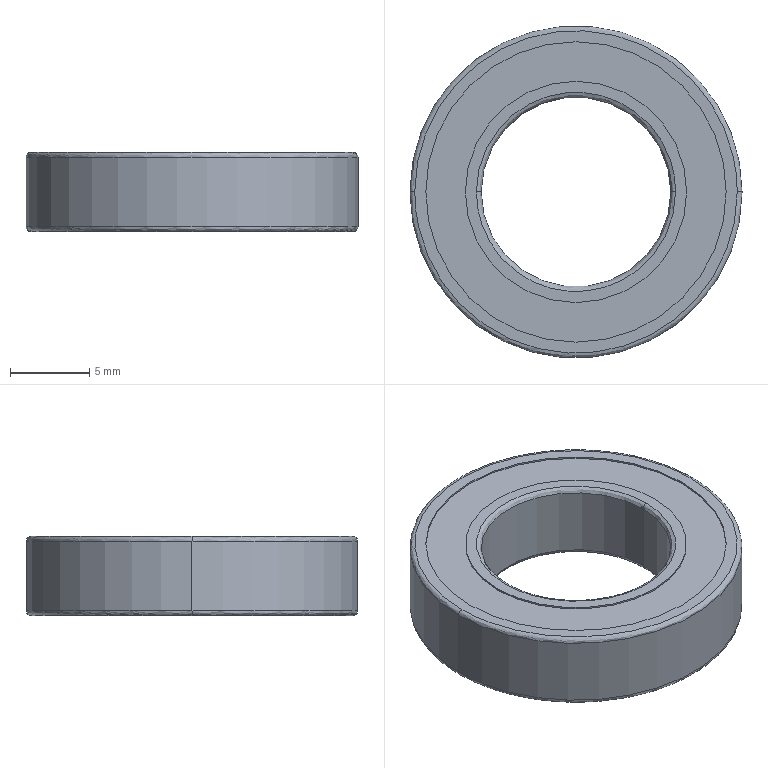Part | SolidWorks | features BaseBody 1 | 1 solid | 26 faces | box 21 x 21 x 5 mm | volume 1137 mm3 | cylinder 12 | spline 8 | plane 6 | commonest cylinder face diameters 14 x4 19 x4 12 x2 21 x2
STEP:
#1=CARTESIAN_POINT('',(-10.2,0.,-5.));
#2=VERTEX_POINT('',#1);
#3=CARTESIAN_POINT('',(10.2,0.,-5.));
#4=VERTEX_POINT('',#3);
#5=CARTESIAN_POINT('',(-10.2,0.,-5.));
#6=CARTESIAN_POINT('',(-10.2,-20.4,-5.));
#7=CARTESIAN_POINT('',(10.2,-20.4,-5.));
#8=CARTESIAN_POINT('',(10.2,0.,-5.));
#9=(BOUNDED_CURVE()B_SPLINE_CURVE(3,(#5,#6,#7,#8),.UNSPECIFIED.,.F.,.F.)B_SPLINE_CURVE_WITH_KNOTS((4,4),(0.,0.5),.UNSPECIFIED.)CURVE()GEOMETRIC_REPRESENTATION_ITEM()RATIONAL_B_SPLINE_CURVE((1.,0.3333,0.3333,1.))REPRESENTATION_ITEM(''));
#10=EDGE_CURVE('',#2,#4,#9,.T.);
#11=ORIENTED_EDGE('',*,*,#10,.T.);
#12=CARTESIAN_POINT('',(10.5,0.,-4.7));
#13=VERTEX_POINT('',#12);
#14=CARTESIAN_POINT('',(10.2,0.,-4.7));
#15=DIRECTION('',(0.,-1.,0.));
#16=DIRECTION('',(1.,0.,0.));
#17=AXIS2_PLACEMENT_3D('',#14,#15,#16);
#18=CIRCLE('',#17,0.3);
#19=EDGE_CURVE('',#4,#13,#18,.T.);
#20=ORIENTED_EDGE('',*,*,#19,.T.);
#21=CARTESIAN_POINT('',(-10.5,0.,-4.7));
#22=VERTEX_POINT('',#21);
#23=CARTESIAN_POINT('',(0.,0.,-4.7));
#24=DIRECTION('',(0.,0.,1.));
#25=DIRECTION('',(1.,0.,0.));
#26=AXIS2_PLACEMENT_3D('',#23,#24,#25);
#27=CIRCLE('',#26,10.5);
#28=EDGE_CURVE('',#22,#13,#27,.T.);
#29=ORIENTED_EDGE('',*,*,#28,.F.);
#30=CARTESIAN_POINT('',(-10.2,0.,-4.7));
#31=DIRECTION('',(0.,1.,0.));
#32=DIRECTION('',(-1.,0.,0.));
#33=AXIS2_PLACEMENT_3D('',#30,#31,#32);
#34=CIRCLE('',#33,0.3);
#35=EDGE_CURVE('',#2,#22,#34,.T.);
#36=ORIENTED_EDGE('',*,*,#35,.F.);
#37=EDGE_LOOP('',(#11,#20,#29,#36));
#38=FACE_OUTER_BOUND('',#37,.T.);
#39=CARTESIAN_POINT('',(10.2,0.,-5.));
#40=CARTESIAN_POINT('',(10.2,-20.4,-5.));
#41=CARTESIAN_POINT('',(-10.2,-20.4,-5.));
#42=CARTESIAN_POINT('',(-10.2,0.,-5.));
#43=CARTESIAN_POINT('',(10.376,0.,-5.));
#44=CARTESIAN_POINT('',(10.376,-20.751,-5.));
#45=CARTESIAN_POINT('',(-10.376,-20.751,-5.));
#46=CARTESIAN_POINT('',(-10.376,0.,-5.));
#47=CARTESIAN_POINT('',(10.5,0.,-4.876));
#48=CARTESIAN_POINT('',(10.5,-21.,-4.876));
#49=CARTESIAN_POINT('',(-10.5,-21.,-4.876));
#50=CARTESIAN_POINT('',(-10.5,0.,-4.876));
#51=CARTESIAN_POINT('',(10.5,0.,-4.7));
#52=CARTESIAN_POINT('',(10.5,-21.,-4.7));
#53=CARTESIAN_POINT('',(-10.5,-21.,-4.7));
#54=CARTESIAN_POINT('',(-10.5,0.,-4.7));
#55=(BOUNDED_SURFACE()B_SPLINE_SURFACE(3,3,((#39,#40,#41,#42),(#43,#44,#45,#46),(#47,#48,#49,#50),(#51,#52,#53,#54)),.UNSPECIFIED.,.F.,.F.,.F.)B_SPLINE_SURFACE_WITH_KNOTS((4,4),(4,4),(0.,1.),(0.,1.),.UNSPECIFIED.)GEOMETRIC_REPRESENTATION_ITEM()RATIONAL_B_SPLINE_SURFACE(((1.,0.3333,0.3333,1.),(0.8047,0.2682,0.2682,0.8047),(0.8047,0.2682,0.2682,0.8047),(1.,0.3333,0.3333,1.)))REPRESENTATION_ITEM('')SURFACE());
#56=ADVANCED_FACE('',(#38),#55,.T.);
#57=CARTESIAN_POINT('',(10.5,0.,-0.3));
#58=VERTEX_POINT('',#57);
#59=CARTESIAN_POINT('',(-10.5,0.,-0.3));
#60=VERTEX_POINT('',#59);
#61=CARTESIAN_POINT('',(0.,0.,-0.3));
#62=DIRECTION('',(0.,0.,-1.));
#63=DIRECTION('',(1.,0.,0.));
#64=AXIS2_PLACEMENT_3D('',#61,#62,#63);
#65=CIRCLE('',#64,10.5);
#66=EDGE_CURVE('',#58,#60,#65,.T.);
#67=ORIENTED_EDGE('',*,*,#66,.F.);
#68=CARTESIAN_POINT('',(10.2,0.,0.));
#69=VERTEX_POINT('',#68);
#70=CARTESIAN_POINT('',(10.2,0.,-0.3));
#71=DIRECTION('',(0.,-1.,0.));
#72=DIRECTION('',(1.,0.,0.));
#73=AXIS2_PLACEMENT_3D('',#70,#71,#72);
#74=CIRCLE('',#73,0.3);
#75=EDGE_CURVE('',#58,#69,#74,.T.);
#76=ORIENTED_EDGE('',*,*,#75,.T.);
#77=CARTESIAN_POINT('',(-10.2,0.,0.));
#78=VERTEX_POINT('',#77);
#79=CARTESIAN_POINT('',(10.2,0.,0.));
#80=CARTESIAN_POINT('',(10.2,-20.4,0.));
#81=CARTESIAN_POINT('',(-10.2,-20.4,0.));
#82=CARTESIAN_POINT('',(-10.2,0.,0.));
#83=(BOUNDED_CURVE()B_SPLINE_CURVE(3,(#79,#80,#81,#82),.UNSPECIFIED.,.F.,.F.)B_SPLINE_CURVE_WITH_KNOTS((4,4),(0.5,1.),.UNSPECIFIED.)CURVE()GEOMETRIC_REPRESENTATION_ITEM()RATIONAL_B_SPLINE_CURVE((1.,0.3333,0.3333,1.))REPRESENTATION_ITEM(''));
#84=EDGE_CURVE('',#69,#78,#83,.T.);
#85=ORIENTED_EDGE('',*,*,#84,.T.);
#86=CARTESIAN_POINT('',(-10.2,0.,-0.3));
#87=DIRECTION('',(0.,1.,0.));
#88=DIRECTION('',(-1.,0.,0.));
#89=AXIS2_PLACEMENT_3D('',#86,#87,#88);
#90=CIRCLE('',#89,0.3);
#91=EDGE_CURVE('',#60,#78,#90,.T.);
#92=ORIENTED_EDGE('',*,*,#91,.F.);
#93=EDGE_LOOP('',(#67,#76,#85,#92));
#94=FACE_OUTER_BOUND('',#93,.T.);
#95=CARTESIAN_POINT('',(10.5,0.,-0.3));
#96=CARTESIAN_POINT('',(10.5,-21.,-0.3));
#97=CARTESIAN_POINT('',(-10.5,-21.,-0.3));
#98=CARTESIAN_POINT('',(-10.5,0.,-0.3));
#99=CARTESIAN_POINT('',(10.5,0.,-0.1243));
#100=CARTESIAN_POINT('',(10.5,-21.,-0.1243));
#101=CARTESIAN_POINT('',(-10.5,-21.,-0.1243));
#102=CARTESIAN_POINT('',(-10.5,0.,-0.1243));
#103=CARTESIAN_POINT('',(10.376,0.,0.));
#104=CARTESIAN_POINT('',(10.376,-20.751,0.));
#105=CARTESIAN_POINT('',(-10.376,-20.751,0.));
#106=CARTESIAN_POINT('',(-10.376,0.,0.));
#107=CARTESIAN_POINT('',(10.2,0.,0.));
#108=CARTESIAN_POINT('',(10.2,-20.4,0.));
#109=CARTESIAN_POINT('',(-10.2,-20.4,0.));
#110=CARTESIAN_POINT('',(-10.2,0.,0.));
#111=(BOUNDED_SURFACE()B_SPLINE_SURFACE(3,3,((#95,#96,#97,#98),(#99,#100,#101,#102),(#103,#104,#105,#106),(#107,#108,#109,#110)),.UNSPECIFIED.,.F.,.F.,.F.)B_SPLINE_SURFACE_WITH_KNOTS((4,4),(4,4),(0.,1.),(0.,1.),.UNSPECIFIED.)GEOMETRIC_REPRESENTATION_ITEM()RATIONAL_B_SPLINE_SURFACE(((1.,0.3333,0.3333,1.),(0.8047,0.2682,0.2682,0.8047),(0.8047,0.2682,0.2682,0.8047),(1.,0.3333,0.3333,1.)))REPRESENTATION_ITEM('')SURFACE());
#112=ADVANCED_FACE('',(#94),#111,.T.);
#113=CARTESIAN_POINT('',(-6.,0.,-4.7));
#114=VERTEX_POINT('',#113);
#115=CARTESIAN_POINT('',(6.,0.,-4.7));
#116=VERTEX_POINT('',#115);
#117=CARTESIAN_POINT('',(0.,0.,-4.7));
#118=DIRECTION('',(0.,0.,1.));
#119=DIRECTION('',(-1.,0.,0.));
#120=AXIS2_PLACEMENT_3D('',#117,#118,#119);
#121=CIRCLE('',#120,6.);
#122=EDGE_CURVE('',#114,#116,#121,.T.);
#123=ORIENTED_EDGE('',*,*,#122,.T.);
#124=CARTESIAN_POINT('',(6.3,0.,-5.));
#125=VERTEX_POINT('',#124);
#126=CARTESIAN_POINT('',(6.3,0.,-4.7));
#127=DIRECTION('',(0.,-1.,0.));
#128=DIRECTION('',(1.,0.,0.));
#129=AXIS2_PLACEMENT_3D('',#126,#127,#128);
#130=CIRCLE('',#129,0.3);
#131=EDGE_CURVE('',#116,#125,#130,.T.);
#132=ORIENTED_EDGE('',*,*,#131,.T.);
#133=CARTESIAN_POINT('',(-6.3,0.,-5.));
#134=VERTEX_POINT('',#133);
#135=CARTESIAN_POINT('',(-6.3,0.,-5.));
#136=CARTESIAN_POINT('',(-6.3,-0.1926,-5.));
#137=CARTESIAN_POINT('',(-6.287,-0.4803,-5.));
#138=CARTESIAN_POINT('',(-6.249,-0.814,-5.));
#139=CARTESIAN_POINT('',(-6.224,-0.9804,-5.));
#140=CARTESIAN_POINT('',(-6.212,-1.052,-5.));
#141=CARTESIAN_POINT('',(-6.203,-1.099,-5.));
#142=CARTESIAN_POINT('',(-6.199,-1.121,-5.));
#143=CARTESIAN_POINT('',(-6.158,-1.347,-5.));
#144=CARTESIAN_POINT('',(-6.088,-1.644,-5.));
#145=CARTESIAN_POINT('',(-5.981,-1.984,-5.));
#146=CARTESIAN_POINT('',(-5.93,-2.128,-5.));
#147=CARTESIAN_POINT('',(-5.895,-2.224,-5.));
#148=CARTESIAN_POINT('',(-5.877,-2.27,-5.));
#149=CARTESIAN_POINT('',(-5.779,-2.517,-5.));
#150=CARTESIAN_POINT('',(-5.648,-2.806,-5.));
#151=CARTESIAN_POINT('',(-5.494,-3.085,-5.));
#152=CARTESIAN_POINT('',(-5.387,-3.268,-5.));
#153=CARTESIAN_POINT('',(-5.333,-3.356,-5.));
#154=CARTESIAN_POINT('',(-5.035,-3.811,-5.));
#155=CARTESIAN_POINT('',(-4.762,-4.147,-5.));
#156=CARTESIAN_POINT('',(-4.301,-4.608,-5.));
#157=CARTESIAN_POINT('',(-4.06,-4.826,-5.));
#158=CARTESIAN_POINT('',(-3.76,-5.057,-5.));
#159=CARTESIAN_POINT('',(-3.627,-5.151,-5.));
#160=CARTESIAN_POINT('',(-3.538,-5.213,-5.));
#161=CARTESIAN_POINT('',(-3.492,-5.244,-5.));
#162=CARTESIAN_POINT('',(-3.269,-5.389,-5.));
#163=CARTESIAN_POINT('',(-2.995,-5.55,-5.));
#164=CARTESIAN_POINT('',(-2.661,-5.712,-5.));
#165=CARTESIAN_POINT('',(-2.516,-5.776,-5.));
#166=CARTESIAN_POINT('',(-2.418,-5.818,-5.));
#167=CARTESIAN_POINT('',(-2.366,-5.839,-5.));
#168=CARTESIAN_POINT('',(-2.129,-5.933,-5.));
#169=CARTESIAN_POINT('',(-1.84,-6.031,-5.));
#170=CARTESIAN_POINT('',(-1.496,-6.121,-5.));
#171=CARTESIAN_POINT('',(-1.322,-6.16,-5.));
#172=CARTESIAN_POINT('',(-1.247,-6.175,-5.));
#173=CARTESIAN_POINT('',(-1.197,-6.185,-5.));
#174=CARTESIAN_POINT('',(-1.17,-6.19,-5.));
#175=CARTESIAN_POINT('',(-0.7678,-6.265,-5.));
#176=CARTESIAN_POINT('',(-0.385,-6.3,-5.));
#177=CARTESIAN_POINT('',(0.1925,-6.3,-5.));
#178=CARTESIAN_POINT('',(0.4802,-6.287,-5.));
#179=CARTESIAN_POINT('',(0.8139,-6.249,-5.));
#180=CARTESIAN_POINT('',(0.9803,-6.224,-5.));
#181=CARTESIAN_POINT('',(1.051,-6.212,-5.));
#182=CARTESIAN_POINT('',(1.099,-6.203,-5.));
#183=CARTESIAN_POINT('',(1.121,-6.199,-5.));
#184=CARTESIAN_POINT('',(1.347,-6.158,-5.));
#185=CARTESIAN_POINT('',(1.644,-6.088,-5.));
#186=CARTESIAN_POINT('',(1.984,-5.981,-5.));
#187=CARTESIAN_POINT('',(2.128,-5.93,-5.));
#188=CARTESIAN_POINT('',(2.224,-5.895,-5.));
#189=CARTESIAN_POINT('',(2.27,-5.877,-5.));
#190=CARTESIAN_POINT('',(2.517,-5.779,-5.));
#191=CARTESIAN_POINT('',(2.806,-5.648,-5.));
#192=CARTESIAN_POINT('',(3.085,-5.494,-5.));
#193=CARTESIAN_POINT('',(3.268,-5.387,-5.));
#194=CARTESIAN_POINT('',(3.356,-5.333,-5.));
#195=CARTESIAN_POINT('',(3.811,-5.035,-5.));
#196=CARTESIAN_POINT('',(4.147,-4.762,-5.));
#197=CARTESIAN_POINT('',(4.608,-4.301,-5.));
#198=CARTESIAN_POINT('',(4.826,-4.06,-5.));
#199=CARTESIAN_POINT('',(5.057,-3.76,-5.));
#200=CARTESIAN_POINT('',(5.151,-3.627,-5.));
#201=CARTESIAN_POINT('',(5.213,-3.538,-5.));
#202=CARTESIAN_POINT('',(5.244,-3.492,-5.));
#203=CARTESIAN_POINT('',(5.389,-3.269,-5.));
#204=CARTESIAN_POINT('',(5.55,-2.995,-5.));
#205=CARTESIAN_POINT('',(5.712,-2.661,-5.));
#206=CARTESIAN_POINT('',(5.776,-2.516,-5.));
#207=CARTESIAN_POINT('',(5.818,-2.418,-5.));
#208=CARTESIAN_POINT('',(5.839,-2.366,-5.));
#209=CARTESIAN_POINT('',(5.933,-2.129,-5.));
#210=CARTESIAN_POINT('',(6.031,-1.84,-5.));
#211=CARTESIAN_POINT('',(6.121,-1.496,-5.));
#212=CARTESIAN_POINT('',(6.16,-1.322,-5.));
#213=CARTESIAN_POINT('',(6.175,-1.247,-5.));
#214=CARTESIAN_POINT('',(6.185,-1.197,-5.));
#215=CARTESIAN_POINT('',(6.19,-1.17,-5.));
#216=CARTESIAN_POINT('',(6.265,-0.7678,-5.));
#217=CARTESIAN_POINT('',(6.3,-0.385,-5.));
#218=CARTESIAN_POINT('',(6.3,0.,-5.));
#219=B_SPLINE_CURVE_WITH_KNOTS('',3,(#135,#136,#137,#138,#139,#140,#141,#142,#143,#144,#145,#146,#147,#148,#149,#150,#151,#152,#153,#154,#155,#156,#157,#158,#159,#160,#161,#162,#163,#164,#165,#166,#167,#168,#169,#170,#171,#172,#173,#174,#175,#176,#177,#178,#179,#180,#181,#182,#183,#184,#185,#186,#187,#188,#189,#190,#191,#192,#193,#194,#195,#196,#197,#198,#199,#200,#201,#202,#203,#204,#205,#206,#207,#208,#209,#210,#211,#212,#213,#214,#215,#216,#217,#218),.UNSPECIFIED.,.F.,.F.,(4,1,1,1,2,2,1,1,2,2,1,2,2,2,1,1,2,2,1,1,2,2,1,1,1,2,2,2,1,1,1,2,2,1,1,2,2,1,2,2,2,1,1,2,2,1,1,2,2,1,1,1,2,2,4),(0.,0.01563,0.02344,0.02734,0.0293,0.03125,0.04688,0.05469,0.05859,0.0625,0.07813,0.08594,0.09375,0.125,0.1406,0.1484,0.1523,0.1563,0.1719,0.1797,0.1836,0.1875,0.2031,0.2109,0.2148,0.2168,0.2188,0.25,0.2656,0.2734,0.2773,0.2793,0.2813,0.2969,0.3047,0.3086,0.3125,0.3281,0.3359,0.3438,0.375,0.3906,0.3984,0.4023,0.4063,0.4219,0.4297,0.4336,0.4375,0.4531,0.4609,0.4648,0.4668,0.4688,0.5),.UNSPECIFIED.);
#220=EDGE_CURVE('',#134,#125,#219,.T.);
#221=ORIENTED_EDGE('',*,*,#220,.F.);
#222=CARTESIAN_POINT('',(-6.3,0.,-4.7));
#223=DIRECTION('',(0.,1.,0.));
#224=DIRECTION('',(-1.,0.,0.));
#225=AXIS2_PLACEMENT_3D('',#222,#223,#224);
#226=CIRCLE('',#225,0.3);
#227=EDGE_CURVE('',#114,#134,#226,.T.);
#228=ORIENTED_EDGE('',*,*,#227,.F.);
#229=EDGE_LOOP('',(#123,#132,#221,#228));
#230=FACE_OUTER_BOUND('',#229,.T.);
#231=CARTESIAN_POINT('',(6.,0.,-4.7));
#232=CARTESIAN_POINT('',(6.,-12.,-4.7));
#233=CARTESIAN_POINT('',(-6.,-12.,-4.7));
#234=CARTESIAN_POINT('',(-6.,0.,-4.7));
#235=CARTESIAN_POINT('',(6.,0.,-4.876));
#236=CARTESIAN_POINT('',(6.,-12.,-4.876));
#237=CARTESIAN_POINT('',(-6.,-12.,-4.876));
#238=CARTESIAN_POINT('',(-6.,0.,-4.876));
#239=CARTESIAN_POINT('',(6.124,0.,-5.));
#240=CARTESIAN_POINT('',(6.124,-12.249,-5.));
#241=CARTESIAN_POINT('',(-6.124,-12.249,-5.));
#242=CARTESIAN_POINT('',(-6.124,0.,-5.));
#243=CARTESIAN_POINT('',(6.3,0.,-5.));
#244=CARTESIAN_POINT('',(6.3,-12.6,-5.));
#245=CARTESIAN_POINT('',(-6.3,-12.6,-5.));
#246=CARTESIAN_POINT('',(-6.3,0.,-5.));
#247=(BOUNDED_SURFACE()B_SPLINE_SURFACE(3,3,((#231,#232,#233,#234),(#235,#236,#237,#238),(#239,#240,#241,#242),(#243,#244,#245,#246)),.UNSPECIFIED.,.F.,.F.,.F.)B_SPLINE_SURFACE_WITH_KNOTS((4,4),(4,4),(0.,1.),(0.,1.),.UNSPECIFIED.)GEOMETRIC_REPRESENTATION_ITEM()RATIONAL_B_SPLINE_SURFACE(((1.,0.3333,0.3333,1.),(0.8047,0.2682,0.2682,0.8047),(0.8047,0.2682,0.2682,0.8047),(1.,0.3333,0.3333,1.)))REPRESENTATION_ITEM('')SURFACE());
#248=ADVANCED_FACE('',(#230),#247,.T.);
#249=CARTESIAN_POINT('',(6.3,0.,0.));
#250=VERTEX_POINT('',#249);
#251=CARTESIAN_POINT('',(-6.3,0.,0.));
#252=VERTEX_POINT('',#251);
#253=CARTESIAN_POINT('',(6.3,0.,0.));
#254=CARTESIAN_POINT('',(6.3,-0.1925,0.));
#255=CARTESIAN_POINT('',(6.287,-0.4802,0.));
#256=CARTESIAN_POINT('',(6.249,-0.8139,0.));
#257=CARTESIAN_POINT('',(6.224,-0.9803,0.));
#258=CARTESIAN_POINT('',(6.212,-1.051,0.));
#259=CARTESIAN_POINT('',(6.203,-1.099,0.));
#260=CARTESIAN_POINT('',(6.199,-1.121,0.));
#261=CARTESIAN_POINT('',(6.158,-1.347,0.));
#262=CARTESIAN_POINT('',(6.088,-1.644,0.));
#263=CARTESIAN_POINT('',(5.981,-1.984,0.));
#264=CARTESIAN_POINT('',(5.93,-2.128,0.));
#265=CARTESIAN_POINT('',(5.895,-2.224,0.));
#266=CARTESIAN_POINT('',(5.877,-2.27,0.));
#267=CARTESIAN_POINT('',(5.779,-2.517,0.));
#268=CARTESIAN_POINT('',(5.648,-2.806,0.));
#269=CARTESIAN_POINT('',(5.494,-3.085,0.));
#270=CARTESIAN_POINT('',(5.387,-3.268,0.));
#271=CARTESIAN_POINT('',(5.333,-3.356,0.));
#272=CARTESIAN_POINT('',(5.035,-3.811,0.));
#273=CARTESIAN_POINT('',(4.762,-4.147,0.));
#274=CARTESIAN_POINT('',(4.301,-4.608,0.));
#275=CARTESIAN_POINT('',(4.06,-4.826,0.));
#276=CARTESIAN_POINT('',(3.76,-5.057,0.));
#277=CARTESIAN_POINT('',(3.627,-5.151,0.));
#278=CARTESIAN_POINT('',(3.538,-5.213,0.));
#279=CARTESIAN_POINT('',(3.492,-5.244,0.));
#280=CARTESIAN_POINT('',(3.269,-5.389,0.));
#281=CARTESIAN_POINT('',(2.995,-5.55,0.));
#282=CARTESIAN_POINT('',(2.661,-5.712,0.));
#283=CARTESIAN_POINT('',(2.516,-5.776,0.));
#284=CARTESIAN_POINT('',(2.418,-5.818,0.));
#285=CARTESIAN_POINT('',(2.366,-5.839,0.));
#286=CARTESIAN_POINT('',(2.129,-5.933,0.));
#287=CARTESIAN_POINT('',(1.84,-6.031,0.));
#288=CARTESIAN_POINT('',(1.496,-6.121,0.));
#289=CARTESIAN_POINT('',(1.322,-6.16,0.));
#290=CARTESIAN_POINT('',(1.247,-6.175,0.));
#291=CARTESIAN_POINT('',(1.197,-6.185,0.));
#292=CARTESIAN_POINT('',(1.17,-6.19,0.));
#293=CARTESIAN_POINT('',(0.7678,-6.265,0.));
#294=CARTESIAN_POINT('',(0.385,-6.3,0.));
#295=CARTESIAN_POINT('',(-0.1925,-6.3,0.));
#296=CARTESIAN_POINT('',(-0.4802,-6.287,0.));
#297=CARTESIAN_POINT('',(-0.8139,-6.249,0.));
#298=CARTESIAN_POINT('',(-0.9803,-6.224,0.));
#299=CARTESIAN_POINT('',(-1.051,-6.212,0.));
#300=CARTESIAN_POINT('',(-1.099,-6.203,0.));
#301=CARTESIAN_POINT('',(-1.121,-6.199,0.));
#302=CARTESIAN_POINT('',(-1.347,-6.158,0.));
#303=CARTESIAN_POINT('',(-1.644,-6.088,0.));
#304=CARTESIAN_POINT('',(-1.984,-5.981,0.));
#305=CARTESIAN_POINT('',(-2.128,-5.93,0.));
#306=CARTESIAN_POINT('',(-2.224,-5.895,0.));
#307=CARTESIAN_POINT('',(-2.27,-5.877,0.));
#308=CARTESIAN_POINT('',(-2.517,-5.779,0.));
#309=CARTESIAN_POINT('',(-2.806,-5.648,0.));
#310=CARTESIAN_POINT('',(-3.085,-5.494,0.));
#311=CARTESIAN_POINT('',(-3.268,-5.387,0.));
#312=CARTESIAN_POINT('',(-3.356,-5.333,0.));
#313=CARTESIAN_POINT('',(-3.811,-5.035,0.));
#314=CARTESIAN_POINT('',(-4.147,-4.762,0.));
#315=CARTESIAN_POINT('',(-4.608,-4.301,0.));
#316=CARTESIAN_POINT('',(-4.826,-4.06,0.));
#317=CARTESIAN_POINT('',(-5.057,-3.76,0.));
#318=CARTESIAN_POINT('',(-5.151,-3.627,0.));
#319=CARTESIAN_POINT('',(-5.213,-3.538,0.));
#320=CARTESIAN_POINT('',(-5.244,-3.492,0.));
#321=CARTESIAN_POINT('',(-5.389,-3.269,0.));
#322=CARTESIAN_POINT('',(-5.55,-2.995,0.));
#323=CARTESIAN_POINT('',(-5.712,-2.661,0.));
#324=CARTESIAN_POINT('',(-5.776,-2.516,0.));
#325=CARTESIAN_POINT('',(-5.818,-2.418,0.));
#326=CARTESIAN_POINT('',(-5.839,-2.366,0.));
#327=CARTESIAN_POINT('',(-5.933,-2.129,0.));
#328=CARTESIAN_POINT('',(-6.031,-1.84,0.));
#329=CARTESIAN_POINT('',(-6.121,-1.496,0.));
#330=CARTESIAN_POINT('',(-6.16,-1.322,0.));
#331=CARTESIAN_POINT('',(-6.175,-1.247,0.));
#332=CARTESIAN_POINT('',(-6.185,-1.197,0.));
#333=CARTESIAN_POINT('',(-6.19,-1.17,0.));
#334=CARTESIAN_POINT('',(-6.265,-0.7676,0.));
#335=CARTESIAN_POINT('',(-6.3,-0.3855,0.));
#336=CARTESIAN_POINT('',(-6.3,0.,0.));
#337=B_SPLINE_CURVE_WITH_KNOTS('',3,(#253,#254,#255,#256,#257,#258,#259,#260,#261,#262,#263,#264,#265,#266,#267,#268,#269,#270,#271,#272,#273,#274,#275,#276,#277,#278,#279,#280,#281,#282,#283,#284,#285,#286,#287,#288,#289,#290,#291,#292,#293,#294,#295,#296,#297,#298,#299,#300,#301,#302,#303,#304,#305,#306,#307,#308,#309,#310,#311,#312,#313,#314,#315,#316,#317,#318,#319,#320,#321,#322,#323,#324,#325,#326,#327,#328,#329,#330,#331,#332,#333,#334,#335,#336),.UNSPECIFIED.,.F.,.F.,(4,1,1,1,2,2,1,1,2,2,1,2,2,2,1,1,2,2,1,1,2,2,1,1,1,2,2,2,1,1,1,2,2,1,1,2,2,1,2,2,2,1,1,2,2,1,1,2,2,1,1,1,2,2,4),(0.5,0.5156,0.5234,0.5273,0.5293,0.5313,0.5469,0.5547,0.5586,0.5625,0.5781,0.5859,0.5938,0.625,0.6406,0.6484,0.6523,0.6563,0.6719,0.6797,0.6836,0.6875,0.7031,0.7109,0.7148,0.7168,0.7188,0.75,0.7656,0.7734,0.7773,0.7793,0.7813,0.7969,0.8047,0.8086,0.8125,0.8281,0.8359,0.8438,0.875,0.8906,0.8984,0.9023,0.9063,0.9219,0.9297,0.9336,0.9375,0.9531,0.9609,0.9648,0.9668,0.9688,1.),.UNSPECIFIED.);
#338=EDGE_CURVE('',#250,#252,#337,.T.);
#339=ORIENTED_EDGE('',*,*,#338,.F.);
#340=CARTESIAN_POINT('',(6.,0.,-0.3));
#341=VERTEX_POINT('',#340);
#342=CARTESIAN_POINT('',(6.3,0.,-0.3));
#343=DIRECTION('',(0.,-1.,0.));
#344=DIRECTION('',(1.,0.,0.));
#345=AXIS2_PLACEMENT_3D('',#342,#343,#344);
#346=CIRCLE('',#345,0.3);
#347=EDGE_CURVE('',#250,#341,#346,.T.);
#348=ORIENTED_EDGE('',*,*,#347,.T.);
#349=CARTESIAN_POINT('',(-6.,0.,-0.3));
#350=VERTEX_POINT('',#349);
#351=CARTESIAN_POINT('',(0.,0.,-0.3));
#352=DIRECTION('',(0.,0.,-1.));
#353=DIRECTION('',(-1.,0.,0.));
#354=AXIS2_PLACEMENT_3D('',#351,#352,#353);
#355=CIRCLE('',#354,6.);
#356=EDGE_CURVE('',#341,#350,#355,.T.);
#357=ORIENTED_EDGE('',*,*,#356,.T.);
#358=CARTESIAN_POINT('',(-6.3,0.,-0.3));
#359=DIRECTION('',(0.,1.,0.));
#360=DIRECTION('',(-1.,0.,0.));
#361=AXIS2_PLACEMENT_3D('',#358,#359,#360);
#362=CIRCLE('',#361,0.3);
#363=EDGE_CURVE('',#252,#350,#362,.T.);
#364=ORIENTED_EDGE('',*,*,#363,.F.);
#365=EDGE_LOOP('',(#339,#348,#357,#364));
#366=FACE_OUTER_BOUND('',#365,.T.);
#367=CARTESIAN_POINT('',(6.3,0.,0.));
#368=CARTESIAN_POINT('',(6.3,-12.6,0.));
#369=CARTESIAN_POINT('',(-6.3,-12.6,0.));
#370=CARTESIAN_POINT('',(-6.3,0.,0.));
#371=CARTESIAN_POINT('',(6.124,0.,0.));
#372=CARTESIAN_POINT('',(6.124,-12.249,0.));
#373=CARTESIAN_POINT('',(-6.124,-12.249,0.));
#374=CARTESIAN_POINT('',(-6.124,0.,0.));
#375=CARTESIAN_POINT('',(6.,0.,-0.1243));
#376=CARTESIAN_POINT('',(6.,-12.,-0.1243));
#377=CARTESIAN_POINT('',(-6.,-12.,-0.1243));
#378=CARTESIAN_POINT('',(-6.,0.,-0.1243));
#379=CARTESIAN_POINT('',(6.,0.,-0.3));
#380=CARTESIAN_POINT('',(6.,-12.,-0.3));
#381=CARTESIAN_POINT('',(-6.,-12.,-0.3));
#382=CARTESIAN_POINT('',(-6.,0.,-0.3));
#383=(BOUNDED_SURFACE()B_SPLINE_SURFACE(3,3,((#367,#368,#369,#370),(#371,#372,#373,#374),(#375,#376,#377,#378),(#379,#380,#381,#382)),.UNSPECIFIED.,.F.,.F.,.F.)B_SPLINE_SURFACE_WITH_KNOTS((4,4),(4,4),(0.,1.),(0.,1.),.UNSPECIFIED.)GEOMETRIC_REPRESENTATION_ITEM()RATIONAL_B_SPLINE_SURFACE(((1.,0.3333,0.3333,1.),(0.8047,0.2682,0.2682,0.8047),(0.8047,0.2682,0.2682,0.8047),(1.,0.3333,0.3333,1.)))REPRESENTATION_ITEM('')SURFACE());
#384=ADVANCED_FACE('',(#366),#383,.T.);
#385=CARTESIAN_POINT('',(0.,0.,-4.7));
#386=DIRECTION('',(0.,0.,1.));
#387=DIRECTION('',(1.,0.,0.));
#388=AXIS2_PLACEMENT_3D('',#385,#386,#387);
#389=CIRCLE('',#388,10.5);
#390=EDGE_CURVE('',#13,#22,#389,.T.);
#391=ORIENTED_EDGE('',*,*,#390,.T.);
#392=CARTESIAN_POINT('',(-10.5,0.,-5.));
#393=DIRECTION('',(0.,0.,1.));
#394=VECTOR('',#393,1000.);
#395=LINE('',#392,#394);
#396=EDGE_CURVE('',#22,#60,#395,.T.);
#397=ORIENTED_EDGE('',*,*,#396,.T.);
#398=CARTESIAN_POINT('',(0.,0.,-0.3));
#399=DIRECTION('',(0.,0.,-1.));
#400=DIRECTION('',(1.,0.,0.));
#401=AXIS2_PLACEMENT_3D('',#398,#399,#400);
#402=CIRCLE('',#401,10.5);
#403=EDGE_CURVE('',#60,#58,#402,.T.);
#404=ORIENTED_EDGE('',*,*,#403,.T.);
#405=CARTESIAN_POINT('',(10.5,0.,-5.));
#406=DIRECTION('',(0.,0.,1.));
#407=VECTOR('',#406,1000.);
#408=LINE('',#405,#407);
#409=EDGE_CURVE('',#13,#58,#408,.T.);
#410=ORIENTED_EDGE('',*,*,#409,.F.);
#411=EDGE_LOOP('',(#391,#397,#404,#410));
#412=FACE_OUTER_BOUND('',#411,.T.);
#413=CARTESIAN_POINT('',(0.,0.,-5.));
#414=DIRECTION('',(0.,0.,1.));
#415=DIRECTION('',(1.,0.,0.));
#416=AXIS2_PLACEMENT_3D('',#413,#414,#415);
#417=CYLINDRICAL_SURFACE('',#416,10.5);
#418=ADVANCED_FACE('',(#412),#417,.T.);
#419=CARTESIAN_POINT('',(-9.5,0.,-5.));
#420=VERTEX_POINT('',#419);
#421=CARTESIAN_POINT('',(9.5,0.,-5.));
#422=VERTEX_POINT('',#421);
#423=CARTESIAN_POINT('',(0.,0.,-5.));
#424=DIRECTION('',(0.,0.,1.));
#425=DIRECTION('',(1.,0.,0.));
#426=AXIS2_PLACEMENT_3D('',#423,#424,#425);
#427=CIRCLE('',#426,9.5);
#428=EDGE_CURVE('',#420,#422,#427,.T.);
#429=ORIENTED_EDGE('',*,*,#428,.F.);
#430=CARTESIAN_POINT('',(-9.5,0.,-4.9));
#431=VERTEX_POINT('',#430);
#432=CARTESIAN_POINT('',(-9.5,0.,-5.));
#433=DIRECTION('',(0.,0.,1.));
#434=VECTOR('',#433,1000.);
#435=LINE('',#432,#434);
#436=EDGE_CURVE('',#420,#431,#435,.T.);
#437=ORIENTED_EDGE('',*,*,#436,.T.);
#438=CARTESIAN_POINT('',(9.5,0.,-4.9));
#439=VERTEX_POINT('',#438);
#440=CARTESIAN_POINT('',(0.,0.,-4.9));
#441=DIRECTION('',(0.,0.,-1.));
#442=DIRECTION('',(1.,0.,0.));
#443=AXIS2_PLACEMENT_3D('',#440,#441,#442);
#444=CIRCLE('',#443,9.5);
#445=EDGE_CURVE('',#439,#431,#444,.T.);
#446=ORIENTED_EDGE('',*,*,#445,.F.);
#447=CARTESIAN_POINT('',(9.5,0.,-5.));
#448=DIRECTION('',(0.,0.,1.));
#449=VECTOR('',#448,1000.);
#450=LINE('',#447,#449);
#451=EDGE_CURVE('',#422,#439,#450,.T.);
#452=ORIENTED_EDGE('',*,*,#451,.F.);
#453=EDGE_LOOP('',(#429,#437,#446,#452));
#454=FACE_OUTER_BOUND('',#453,.T.);
#455=CARTESIAN_POINT('',(0.,0.,-5.));
#456=DIRECTION('',(0.,0.,1.));
#457=DIRECTION('',(1.,0.,0.));
#458=AXIS2_PLACEMENT_3D('',#455,#456,#457);
#459=CYLINDRICAL_SURFACE('',#458,9.5);
#460=ADVANCED_FACE('',(#454),#459,.F.);
#461=CARTESIAN_POINT('',(-9.5,0.,-0.1));
#462=VERTEX_POINT('',#461);
#463=CARTESIAN_POINT('',(9.5,0.,-0.1));
#464=VERTEX_POINT('',#463);
#465=CARTESIAN_POINT('',(0.,0.,-0.1));
#466=DIRECTION('',(0.,0.,1.));
#467=DIRECTION('',(1.,0.,0.));
#468=AXIS2_PLACEMENT_3D('',#465,#466,#467);
#469=CIRCLE('',#468,9.5);
#470=EDGE_CURVE('',#462,#464,#469,.T.);
#471=ORIENTED_EDGE('',*,*,#470,.F.);
#472=CARTESIAN_POINT('',(-9.5,0.,0.));
#473=VERTEX_POINT('',#472);
#474=CARTESIAN_POINT('',(-9.5,0.,-5.));
#475=DIRECTION('',(0.,0.,1.));
#476=VECTOR('',#475,1000.);
#477=LINE('',#474,#476);
#478=EDGE_CURVE('',#462,#473,#477,.T.);
#479=ORIENTED_EDGE('',*,*,#478,.T.);
#480=CARTESIAN_POINT('',(9.5,0.,0.));
#481=VERTEX_POINT('',#480);
#482=CARTESIAN_POINT('',(0.,0.,0.));
#483=DIRECTION('',(0.,0.,-1.));
#484=DIRECTION('',(1.,0.,0.));
#485=AXIS2_PLACEMENT_3D('',#482,#483,#484);
#486=CIRCLE('',#485,9.5);
#487=EDGE_CURVE('',#481,#473,#486,.T.);
#488=ORIENTED_EDGE('',*,*,#487,.F.);
#489=CARTESIAN_POINT('',(9.5,0.,-5.));
#490=DIRECTION('',(0.,0.,1.));
#491=VECTOR('',#490,1000.);
#492=LINE('',#489,#491);
#493=EDGE_CURVE('',#464,#481,#492,.T.);
#494=ORIENTED_EDGE('',*,*,#493,.F.);
#495=EDGE_LOOP('',(#471,#479,#488,#494));
#496=FACE_OUTER_BOUND('',#495,.T.);
#497=CARTESIAN_POINT('',(0.,0.,-5.));
#498=DIRECTION('',(0.,0.,1.));
#499=DIRECTION('',(1.,0.,0.));
#500=AXIS2_PLACEMENT_3D('',#497,#498,#499);
#501=CYLINDRICAL_SURFACE('',#500,9.5);
#502=ADVANCED_FACE('',(#496),#501,.F.);
#503=CARTESIAN_POINT('',(7.,0.,-5.));
#504=VERTEX_POINT('',#503);
#505=CARTESIAN_POINT('',(-7.,0.,-5.));
#506=VERTEX_POINT('',#505);
#507=CARTESIAN_POINT('',(0.,0.,-5.));
#508=DIRECTION('',(0.,0.,1.));
#509=DIRECTION('',(1.,0.,0.));
#510=AXIS2_PLACEMENT_3D('',#507,#508,#509);
#511=CIRCLE('',#510,7.);
#512=EDGE_CURVE('',#504,#506,#511,.T.);
#513=ORIENTED_EDGE('',*,*,#512,.T.);
#514=CARTESIAN_POINT('',(-7.,0.,-4.9));
#515=VERTEX_POINT('',#514);
#516=CARTESIAN_POINT('',(-7.,0.,-5.));
#517=DIRECTION('',(0.,0.,1.));
#518=VECTOR('',#517,1000.);
#519=LINE('',#516,#518);
#520=EDGE_CURVE('',#506,#515,#519,.T.);
#521=ORIENTED_EDGE('',*,*,#520,.T.);
#522=CARTESIAN_POINT('',(7.,0.,-4.9));
#523=VERTEX_POINT('',#522);
#524=CARTESIAN_POINT('',(0.,0.,-4.9));
#525=DIRECTION('',(0.,0.,1.));
#526=DIRECTION('',(1.,0.,0.));
#527=AXIS2_PLACEMENT_3D('',#524,#525,#526);
#528=CIRCLE('',#527,7.);
#529=EDGE_CURVE('',#523,#515,#528,.T.);
#530=ORIENTED_EDGE('',*,*,#529,.F.);
#531=CARTESIAN_POINT('',(7.,0.,-5.));
#532=DIRECTION('',(0.,0.,1.));
#533=VECTOR('',#532,1000.);
#534=LINE('',#531,#533);
#535=EDGE_CURVE('',#504,#523,#534,.T.);
#536=ORIENTED_EDGE('',*,*,#535,.F.);
#537=EDGE_LOOP('',(#513,#521,#530,#536));
#538=FACE_OUTER_BOUND('',#537,.T.);
#539=CARTESIAN_POINT('',(0.,0.,-5.));
#540=DIRECTION('',(0.,0.,1.));
#541=DIRECTION('',(1.,0.,0.));
#542=AXIS2_PLACEMENT_3D('',#539,#540,#541);
#543=CYLINDRICAL_SURFACE('',#542,7.);
#544=ADVANCED_FACE('',(#538),#543,.T.);
#545=CARTESIAN_POINT('',(-7.,0.,-0.1));
#546=VERTEX_POINT('',#545);
#547=CARTESIAN_POINT('',(7.,0.,-0.1));
#548=VERTEX_POINT('',#547);
#549=CARTESIAN_POINT('',(0.,0.,-0.1));
#550=DIRECTION('',(0.,0.,-1.));
#551=DIRECTION('',(1.,0.,0.));
#552=AXIS2_PLACEMENT_3D('',#549,#550,#551);
#553=CIRCLE('',#552,7.);
#554=EDGE_CURVE('',#546,#548,#553,.T.);
#555=ORIENTED_EDGE('',*,*,#554,.F.);
#556=CARTESIAN_POINT('',(-7.,0.,0.));
#557=VERTEX_POINT('',#556);
#558=CARTESIAN_POINT('',(-7.,0.,-5.));
#559=DIRECTION('',(0.,0.,1.));
#560=VECTOR('',#559,1000.);
#561=LINE('',#558,#560);
#562=EDGE_CURVE('',#546,#557,#561,.T.);
#563=ORIENTED_EDGE('',*,*,#562,.T.);
#564=CARTESIAN_POINT('',(7.,0.,0.));
#565=VERTEX_POINT('',#564);
#566=CARTESIAN_POINT('',(0.,0.,0.));
#567=DIRECTION('',(0.,0.,-1.));
#568=DIRECTION('',(1.,0.,0.));
#569=AXIS2_PLACEMENT_3D('',#566,#567,#568);
#570=CIRCLE('',#569,7.);
#571=EDGE_CURVE('',#557,#565,#570,.T.);
#572=ORIENTED_EDGE('',*,*,#571,.T.);
#573=CARTESIAN_POINT('',(7.,0.,-5.));
#574=DIRECTION('',(0.,0.,1.));
#575=VECTOR('',#574,1000.);
#576=LINE('',#573,#575);
#577=EDGE_CURVE('',#548,#565,#576,.T.);
#578=ORIENTED_EDGE('',*,*,#577,.F.);
#579=EDGE_LOOP('',(#555,#563,#572,#578));
#580=FACE_OUTER_BOUND('',#579,.T.);
#581=CARTESIAN_POINT('',(0.,0.,-5.));
#582=DIRECTION('',(0.,0.,1.));
#583=DIRECTION('',(1.,0.,0.));
#584=AXIS2_PLACEMENT_3D('',#581,#582,#583);
#585=CYLINDRICAL_SURFACE('',#584,7.);
#586=ADVANCED_FACE('',(#580),#585,.T.);
#587=ORIENTED_EDGE('',*,*,#122,.F.);
#588=CARTESIAN_POINT('',(-6.,0.,-5.));
#589=DIRECTION('',(0.,0.,1.));
#590=VECTOR('',#589,1000.);
#591=LINE('',#588,#590);
#592=EDGE_CURVE('',#114,#350,#591,.T.);
#593=ORIENTED_EDGE('',*,*,#592,.T.);
#594=ORIENTED_EDGE('',*,*,#356,.F.);
#595=CARTESIAN_POINT('',(6.,0.,-5.));
#596=DIRECTION('',(0.,0.,1.));
#597=VECTOR('',#596,1000.);
#598=LINE('',#595,#597);
#599=EDGE_CURVE('',#116,#341,#598,.T.);
#600=ORIENTED_EDGE('',*,*,#599,.F.);
#601=EDGE_LOOP('',(#587,#593,#594,#600));
#602=FACE_OUTER_BOUND('',#601,.T.);
#603=CARTESIAN_POINT('',(0.,0.,-5.));
#604=DIRECTION('',(0.,0.,1.));
#605=DIRECTION('',(1.,0.,0.));
#606=AXIS2_PLACEMENT_3D('',#603,#604,#605);
#607=CYLINDRICAL_SURFACE('',#606,6.);
#608=ADVANCED_FACE('',(#602),#607,.F.);
#609=ORIENTED_EDGE('',*,*,#396,.F.);
#610=ORIENTED_EDGE('',*,*,#28,.T.);
#611=ORIENTED_EDGE('',*,*,#409,.T.);
#612=ORIENTED_EDGE('',*,*,#66,.T.);
#613=EDGE_LOOP('',(#609,#610,#611,#612));
#614=FACE_OUTER_BOUND('',#613,.T.);
#615=CARTESIAN_POINT('',(0.,0.,-5.));
#616=DIRECTION('',(0.,0.,1.));
#617=DIRECTION('',(1.,0.,0.));
#618=AXIS2_PLACEMENT_3D('',#615,#616,#617);
#619=CYLINDRICAL_SURFACE('',#618,10.5);
#620=ADVANCED_FACE('',(#614),#619,.T.);
#621=ORIENTED_EDGE('',*,*,#19,.F.);
#622=CARTESIAN_POINT('',(10.2,0.,-5.));
#623=CARTESIAN_POINT('',(10.2,20.4,-5.));
#624=CARTESIAN_POINT('',(-10.2,20.4,-5.));
#625=CARTESIAN_POINT('',(-10.2,0.,-5.));
#626=(BOUNDED_CURVE()B_SPLINE_CURVE(3,(#622,#623,#624,#625),.UNSPECIFIED.,.F.,.F.)B_SPLINE_CURVE_WITH_KNOTS((4,4),(0.5,1.),.UNSPECIFIED.)CURVE()GEOMETRIC_REPRESENTATION_ITEM()RATIONAL_B_SPLINE_CURVE((1.,0.3333,0.3333,1.))REPRESENTATION_ITEM(''));
#627=EDGE_CURVE('',#4,#2,#626,.T.);
#628=ORIENTED_EDGE('',*,*,#627,.T.);
#629=ORIENTED_EDGE('',*,*,#35,.T.);
#630=ORIENTED_EDGE('',*,*,#390,.F.);
#631=EDGE_LOOP('',(#621,#628,#629,#630));
#632=FACE_OUTER_BOUND('',#631,.T.);
#633=CARTESIAN_POINT('',(-10.2,0.,-5.));
#634=CARTESIAN_POINT('',(-10.2,20.4,-5.));
#635=CARTESIAN_POINT('',(10.2,20.4,-5.));
#636=CARTESIAN_POINT('',(10.2,0.,-5.));
#637=CARTESIAN_POINT('',(-10.376,0.,-5.));
#638=CARTESIAN_POINT('',(-10.376,20.751,-5.));
#639=CARTESIAN_POINT('',(10.376,20.751,-5.));
#640=CARTESIAN_POINT('',(10.376,0.,-5.));
#641=CARTESIAN_POINT('',(-10.5,0.,-4.876));
#642=CARTESIAN_POINT('',(-10.5,21.,-4.876));
#643=CARTESIAN_POINT('',(10.5,21.,-4.876));
#644=CARTESIAN_POINT('',(10.5,0.,-4.876));
#645=CARTESIAN_POINT('',(-10.5,0.,-4.7));
#646=CARTESIAN_POINT('',(-10.5,21.,-4.7));
#647=CARTESIAN_POINT('',(10.5,21.,-4.7));
#648=CARTESIAN_POINT('',(10.5,0.,-4.7));
#649=(BOUNDED_SURFACE()B_SPLINE_SURFACE(3,3,((#633,#634,#635,#636),(#637,#638,#639,#640),(#641,#642,#643,#644),(#645,#646,#647,#648)),.UNSPECIFIED.,.F.,.F.,.T.)B_SPLINE_SURFACE_WITH_KNOTS((4,4),(4,4),(0.,1.),(0.,1.),.UNSPECIFIED.)GEOMETRIC_REPRESENTATION_ITEM()RATIONAL_B_SPLINE_SURFACE(((1.,0.3333,0.3333,1.),(0.8047,0.2682,0.2682,0.8047),(0.8047,0.2682,0.2682,0.8047),(1.,0.3333,0.3333,1.)))REPRESENTATION_ITEM('')SURFACE());
#650=ADVANCED_FACE('',(#632),#649,.T.);
#651=ORIENTED_EDGE('',*,*,#75,.F.);
#652=ORIENTED_EDGE('',*,*,#403,.F.);
#653=ORIENTED_EDGE('',*,*,#91,.T.);
#654=CARTESIAN_POINT('',(-10.2,0.,0.));
#655=CARTESIAN_POINT('',(-10.2,20.4,0.));
#656=CARTESIAN_POINT('',(10.2,20.4,0.));
#657=CARTESIAN_POINT('',(10.2,0.,0.));
#658=(BOUNDED_CURVE()B_SPLINE_CURVE(3,(#654,#655,#656,#657),.UNSPECIFIED.,.F.,.F.)B_SPLINE_CURVE_WITH_KNOTS((4,4),(0.,0.5),.UNSPECIFIED.)CURVE()GEOMETRIC_REPRESENTATION_ITEM()RATIONAL_B_SPLINE_CURVE((1.,0.3333,0.3333,1.))REPRESENTATION_ITEM(''));
#659=EDGE_CURVE('',#78,#69,#658,.T.);
#660=ORIENTED_EDGE('',*,*,#659,.T.);
#661=EDGE_LOOP('',(#651,#652,#653,#660));
#662=FACE_OUTER_BOUND('',#661,.T.);
#663=CARTESIAN_POINT('',(-10.5,0.,-0.3));
#664=CARTESIAN_POINT('',(-10.5,21.,-0.3));
#665=CARTESIAN_POINT('',(10.5,21.,-0.3));
#666=CARTESIAN_POINT('',(10.5,0.,-0.3));
#667=CARTESIAN_POINT('',(-10.5,0.,-0.1243));
#668=CARTESIAN_POINT('',(-10.5,21.,-0.1243));
#669=CARTESIAN_POINT('',(10.5,21.,-0.1243));
#670=CARTESIAN_POINT('',(10.5,0.,-0.1243));
#671=CARTESIAN_POINT('',(-10.376,0.,0.));
#672=CARTESIAN_POINT('',(-10.376,20.751,0.));
#673=CARTESIAN_POINT('',(10.376,20.751,0.));
#674=CARTESIAN_POINT('',(10.376,0.,0.));
#675=CARTESIAN_POINT('',(-10.2,0.,0.));
#676=CARTESIAN_POINT('',(-10.2,20.4,0.));
#677=CARTESIAN_POINT('',(10.2,20.4,0.));
#678=CARTESIAN_POINT('',(10.2,0.,0.));
#679=(BOUNDED_SURFACE()B_SPLINE_SURFACE(3,3,((#663,#664,#665,#666),(#667,#668,#669,#670),(#671,#672,#673,#674),(#675,#676,#677,#678)),.UNSPECIFIED.,.F.,.F.,.F.)B_SPLINE_SURFACE_WITH_KNOTS((4,4),(4,4),(0.,1.),(0.,1.),.UNSPECIFIED.)GEOMETRIC_REPRESENTATION_ITEM()RATIONAL_B_SPLINE_SURFACE(((1.,0.3333,0.3333,1.),(0.8047,0.2682,0.2682,0.8047),(0.8047,0.2682,0.2682,0.8047),(1.,0.3333,0.3333,1.)))REPRESENTATION_ITEM('')SURFACE());
#680=ADVANCED_FACE('',(#662),#679,.T.);
#681=CARTESIAN_POINT('',(0.,0.,-5.));
#682=DIRECTION('',(0.,0.,1.));
#683=DIRECTION('',(1.,0.,0.));
#684=AXIS2_PLACEMENT_3D('',#681,#682,#683);
#685=CIRCLE('',#684,9.5);
#686=EDGE_CURVE('',#422,#420,#685,.T.);
#687=ORIENTED_EDGE('',*,*,#686,.T.);
#688=ORIENTED_EDGE('',*,*,#428,.T.);
#689=EDGE_LOOP('',(#687,#688));
#690=FACE_BOUND('',#689,.T.);
#691=ORIENTED_EDGE('',*,*,#10,.F.);
#692=ORIENTED_EDGE('',*,*,#627,.F.);
#693=EDGE_LOOP('',(#691,#692));
#694=FACE_OUTER_BOUND('',#693,.T.);
#695=CARTESIAN_POINT('',(0.,9.5,-5.));
#696=DIRECTION('',(0.,0.,-1.));
#697=DIRECTION('',(-1.,0.,0.));
#698=AXIS2_PLACEMENT_3D('',#695,#696,#697);
#699=PLANE('',#698);
#700=ADVANCED_FACE('',(#690,#694),#699,.T.);
#701=ORIENTED_EDGE('',*,*,#659,.F.);
#702=ORIENTED_EDGE('',*,*,#84,.F.);
#703=EDGE_LOOP('',(#701,#702));
#704=FACE_OUTER_BOUND('',#703,.T.);
#705=ORIENTED_EDGE('',*,*,#487,.T.);
#706=CARTESIAN_POINT('',(0.,0.,0.));
#707=DIRECTION('',(0.,0.,-1.));
#708=DIRECTION('',(1.,0.,0.));
#709=AXIS2_PLACEMENT_3D('',#706,#707,#708);
#710=CIRCLE('',#709,9.5);
#711=EDGE_CURVE('',#473,#481,#710,.T.);
#712=ORIENTED_EDGE('',*,*,#711,.T.);
#713=EDGE_LOOP('',(#705,#712));
#714=FACE_BOUND('',#713,.T.);
#715=CARTESIAN_POINT('',(0.,10.2,0.));
#716=DIRECTION('',(0.,0.,1.));
#717=DIRECTION('',(1.,0.,0.));
#718=AXIS2_PLACEMENT_3D('',#715,#716,#717);
#719=PLANE('',#718);
#720=ADVANCED_FACE('',(#704,#714),#719,.T.);
#721=ORIENTED_EDGE('',*,*,#436,.F.);
#722=ORIENTED_EDGE('',*,*,#686,.F.);
#723=ORIENTED_EDGE('',*,*,#451,.T.);
#724=CARTESIAN_POINT('',(0.,0.,-4.9));
#725=DIRECTION('',(0.,0.,-1.));
#726=DIRECTION('',(1.,0.,0.));
#727=AXIS2_PLACEMENT_3D('',#724,#725,#726);
#728=CIRCLE('',#727,9.5);
#729=EDGE_CURVE('',#431,#439,#728,.T.);
#730=ORIENTED_EDGE('',*,*,#729,.F.);
#731=EDGE_LOOP('',(#721,#722,#723,#730));
#732=FACE_OUTER_BOUND('',#731,.T.);
#733=CARTESIAN_POINT('',(0.,0.,-5.));
#734=DIRECTION('',(0.,0.,1.));
#735=DIRECTION('',(1.,0.,0.));
#736=AXIS2_PLACEMENT_3D('',#733,#734,#735);
#737=CYLINDRICAL_SURFACE('',#736,9.5);
#738=ADVANCED_FACE('',(#732),#737,.F.);
#739=ORIENTED_EDGE('',*,*,#478,.F.);
#740=CARTESIAN_POINT('',(0.,0.,-0.1));
#741=DIRECTION('',(0.,0.,1.));
#742=DIRECTION('',(1.,0.,0.));
#743=AXIS2_PLACEMENT_3D('',#740,#741,#742);
#744=CIRCLE('',#743,9.5);
#745=EDGE_CURVE('',#464,#462,#744,.T.);
#746=ORIENTED_EDGE('',*,*,#745,.F.);
#747=ORIENTED_EDGE('',*,*,#493,.T.);
#748=ORIENTED_EDGE('',*,*,#711,.F.);
#749=EDGE_LOOP('',(#739,#746,#747,#748));
#750=FACE_OUTER_BOUND('',#749,.T.);
#751=CARTESIAN_POINT('',(0.,0.,-5.));
#752=DIRECTION('',(0.,0.,1.));
#753=DIRECTION('',(1.,0.,0.));
#754=AXIS2_PLACEMENT_3D('',#751,#752,#753);
#755=CYLINDRICAL_SURFACE('',#754,9.5);
#756=ADVANCED_FACE('',(#750),#755,.F.);
#757=ORIENTED_EDGE('',*,*,#529,.T.);
#758=CARTESIAN_POINT('',(0.,0.,-4.9));
#759=DIRECTION('',(0.,0.,1.));
#760=DIRECTION('',(1.,0.,0.));
#761=AXIS2_PLACEMENT_3D('',#758,#759,#760);
#762=CIRCLE('',#761,7.);
#763=EDGE_CURVE('',#515,#523,#762,.T.);
#764=ORIENTED_EDGE('',*,*,#763,.T.);
#765=EDGE_LOOP('',(#757,#764));
#766=FACE_BOUND('',#765,.T.);
#767=ORIENTED_EDGE('',*,*,#445,.T.);
#768=ORIENTED_EDGE('',*,*,#729,.T.);
#769=EDGE_LOOP('',(#767,#768));
#770=FACE_OUTER_BOUND('',#769,.T.);
#771=CARTESIAN_POINT('',(0.,7.,-4.9));
#772=DIRECTION('',(0.,0.,-1.));
#773=DIRECTION('',(-1.,0.,0.));
#774=AXIS2_PLACEMENT_3D('',#771,#772,#773);
#775=PLANE('',#774);
#776=ADVANCED_FACE('',(#766,#770),#775,.T.);
#777=ORIENTED_EDGE('',*,*,#745,.T.);
#778=ORIENTED_EDGE('',*,*,#470,.T.);
#779=EDGE_LOOP('',(#777,#778));
#780=FACE_OUTER_BOUND('',#779,.T.);
#781=CARTESIAN_POINT('',(0.,0.,-0.1));
#782=DIRECTION('',(0.,0.,-1.));
#783=DIRECTION('',(1.,0.,0.));
#784=AXIS2_PLACEMENT_3D('',#781,#782,#783);
#785=CIRCLE('',#784,7.);
#786=EDGE_CURVE('',#548,#546,#785,.T.);
#787=ORIENTED_EDGE('',*,*,#786,.T.);
#788=ORIENTED_EDGE('',*,*,#554,.T.);
#789=EDGE_LOOP('',(#787,#788));
#790=FACE_BOUND('',#789,.T.);
#791=CARTESIAN_POINT('',(0.,9.5,-0.1));
#792=DIRECTION('',(0.,0.,1.));
#793=DIRECTION('',(1.,0.,0.));
#794=AXIS2_PLACEMENT_3D('',#791,#792,#793);
#795=PLANE('',#794);
#796=ADVANCED_FACE('',(#780,#790),#795,.T.);
#797=ORIENTED_EDGE('',*,*,#520,.F.);
#798=CARTESIAN_POINT('',(0.,0.,-5.));
#799=DIRECTION('',(0.,0.,1.));
#800=DIRECTION('',(1.,0.,0.));
#801=AXIS2_PLACEMENT_3D('',#798,#799,#800);
#802=CIRCLE('',#801,7.);
#803=EDGE_CURVE('',#506,#504,#802,.T.);
#804=ORIENTED_EDGE('',*,*,#803,.T.);
#805=ORIENTED_EDGE('',*,*,#535,.T.);
#806=ORIENTED_EDGE('',*,*,#763,.F.);
#807=EDGE_LOOP('',(#797,#804,#805,#806));
#808=FACE_OUTER_BOUND('',#807,.T.);
#809=CARTESIAN_POINT('',(0.,0.,-5.));
#810=DIRECTION('',(0.,0.,1.));
#811=DIRECTION('',(1.,0.,0.));
#812=AXIS2_PLACEMENT_3D('',#809,#810,#811);
#813=CYLINDRICAL_SURFACE('',#812,7.);
#814=ADVANCED_FACE('',(#808),#813,.T.);
#815=ORIENTED_EDGE('',*,*,#562,.F.);
#816=ORIENTED_EDGE('',*,*,#786,.F.);
#817=ORIENTED_EDGE('',*,*,#577,.T.);
#818=CARTESIAN_POINT('',(0.,0.,0.));
#819=DIRECTION('',(0.,0.,-1.));
#820=DIRECTION('',(1.,0.,0.));
#821=AXIS2_PLACEMENT_3D('',#818,#819,#820);
#822=CIRCLE('',#821,7.);
#823=EDGE_CURVE('',#565,#557,#822,.T.);
#824=ORIENTED_EDGE('',*,*,#823,.T.);
#825=EDGE_LOOP('',(#815,#816,#817,#824));
#826=FACE_OUTER_BOUND('',#825,.T.);
#827=CARTESIAN_POINT('',(0.,0.,-5.));
#828=DIRECTION('',(0.,0.,1.));
#829=DIRECTION('',(1.,0.,0.));
#830=AXIS2_PLACEMENT_3D('',#827,#828,#829);
#831=CYLINDRICAL_SURFACE('',#830,7.);
#832=ADVANCED_FACE('',(#826),#831,.T.);
#833=ORIENTED_EDGE('',*,*,#220,.T.);
#834=CARTESIAN_POINT('',(6.3,0.,-5.));
#835=CARTESIAN_POINT('',(6.3,0.1925,-5.));
#836=CARTESIAN_POINT('',(6.287,0.4802,-5.));
#837=CARTESIAN_POINT('',(6.249,0.8139,-5.));
#838=CARTESIAN_POINT('',(6.224,0.9803,-5.));
#839=CARTESIAN_POINT('',(6.212,1.051,-5.));
#840=CARTESIAN_POINT('',(6.203,1.099,-5.));
#841=CARTESIAN_POINT('',(6.199,1.121,-5.));
#842=CARTESIAN_POINT('',(6.158,1.347,-5.));
#843=CARTESIAN_POINT('',(6.088,1.644,-5.));
#844=CARTESIAN_POINT('',(5.981,1.984,-5.));
#845=CARTESIAN_POINT('',(5.93,2.128,-5.));
#846=CARTESIAN_POINT('',(5.895,2.224,-5.));
#847=CARTESIAN_POINT('',(5.877,2.27,-5.));
#848=CARTESIAN_POINT('',(5.779,2.517,-5.));
#849=CARTESIAN_POINT('',(5.648,2.806,-5.));
#850=CARTESIAN_POINT('',(5.494,3.085,-5.));
#851=CARTESIAN_POINT('',(5.387,3.268,-5.));
#852=CARTESIAN_POINT('',(5.333,3.356,-5.));
#853=CARTESIAN_POINT('',(5.035,3.811,-5.));
#854=CARTESIAN_POINT('',(4.762,4.147,-5.));
#855=CARTESIAN_POINT('',(4.301,4.608,-5.));
#856=CARTESIAN_POINT('',(4.06,4.826,-5.));
#857=CARTESIAN_POINT('',(3.76,5.057,-5.));
#858=CARTESIAN_POINT('',(3.627,5.151,-5.));
#859=CARTESIAN_POINT('',(3.538,5.213,-5.));
#860=CARTESIAN_POINT('',(3.492,5.244,-5.));
#861=CARTESIAN_POINT('',(3.269,5.389,-5.));
#862=CARTESIAN_POINT('',(2.995,5.55,-5.));
#863=CARTESIAN_POINT('',(2.661,5.712,-5.));
#864=CARTESIAN_POINT('',(2.516,5.776,-5.));
#865=CARTESIAN_POINT('',(2.418,5.818,-5.));
#866=CARTESIAN_POINT('',(2.366,5.839,-5.));
#867=CARTESIAN_POINT('',(2.129,5.933,-5.));
#868=CARTESIAN_POINT('',(1.84,6.031,-5.));
#869=CARTESIAN_POINT('',(1.496,6.121,-5.));
#870=CARTESIAN_POINT('',(1.322,6.16,-5.));
#871=CARTESIAN_POINT('',(1.247,6.175,-5.));
#872=CARTESIAN_POINT('',(1.197,6.185,-5.));
#873=CARTESIAN_POINT('',(1.17,6.19,-5.));
#874=CARTESIAN_POINT('',(0.7678,6.265,-5.));
#875=CARTESIAN_POINT('',(0.385,6.3,-5.));
#876=CARTESIAN_POINT('',(-0.1925,6.3,-5.));
#877=CARTESIAN_POINT('',(-0.4802,6.287,-5.));
#878=CARTESIAN_POINT('',(-0.8139,6.249,-5.));
#879=CARTESIAN_POINT('',(-0.9803,6.224,-5.));
#880=CARTESIAN_POINT('',(-1.051,6.212,-5.));
#881=CARTESIAN_POINT('',(-1.099,6.203,-5.));
#882=CARTESIAN_POINT('',(-1.121,6.199,-5.));
#883=CARTESIAN_POINT('',(-1.347,6.158,-5.));
#884=CARTESIAN_POINT('',(-1.644,6.088,-5.));
#885=CARTESIAN_POINT('',(-1.984,5.981,-5.));
#886=CARTESIAN_POINT('',(-2.128,5.93,-5.));
#887=CARTESIAN_POINT('',(-2.224,5.895,-5.));
#888=CARTESIAN_POINT('',(-2.27,5.877,-5.));
#889=CARTESIAN_POINT('',(-2.517,5.779,-5.));
#890=CARTESIAN_POINT('',(-2.806,5.648,-5.));
#891=CARTESIAN_POINT('',(-3.085,5.494,-5.));
#892=CARTESIAN_POINT('',(-3.268,5.387,-5.));
#893=CARTESIAN_POINT('',(-3.356,5.333,-5.));
#894=CARTESIAN_POINT('',(-3.811,5.035,-5.));
#895=CARTESIAN_POINT('',(-4.147,4.762,-5.));
#896=CARTESIAN_POINT('',(-4.608,4.301,-5.));
#897=CARTESIAN_POINT('',(-4.826,4.06,-5.));
#898=CARTESIAN_POINT('',(-5.057,3.76,-5.));
#899=CARTESIAN_POINT('',(-5.151,3.627,-5.));
#900=CARTESIAN_POINT('',(-5.213,3.538,-5.));
#901=CARTESIAN_POINT('',(-5.244,3.492,-5.));
#902=CARTESIAN_POINT('',(-5.389,3.269,-5.));
#903=CARTESIAN_POINT('',(-5.55,2.995,-5.));
#904=CARTESIAN_POINT('',(-5.712,2.661,-5.));
#905=CARTESIAN_POINT('',(-5.776,2.516,-5.));
#906=CARTESIAN_POINT('',(-5.818,2.418,-5.));
#907=CARTESIAN_POINT('',(-5.839,2.366,-5.));
#908=CARTESIAN_POINT('',(-5.933,2.129,-5.));
#909=CARTESIAN_POINT('',(-6.031,1.84,-5.));
#910=CARTESIAN_POINT('',(-6.121,1.496,-5.));
#911=CARTESIAN_POINT('',(-6.16,1.322,-5.));
#912=CARTESIAN_POINT('',(-6.175,1.247,-5.));
#913=CARTESIAN_POINT('',(-6.185,1.197,-5.));
#914=CARTESIAN_POINT('',(-6.19,1.17,-5.));
#915=CARTESIAN_POINT('',(-6.265,0.7676,-5.));
#916=CARTESIAN_POINT('',(-6.3,0.3855,-5.));
#917=CARTESIAN_POINT('',(-6.3,0.,-5.));
#918=B_SPLINE_CURVE_WITH_KNOTS('',3,(#834,#835,#836,#837,#838,#839,#840,#841,#842,#843,#844,#845,#846,#847,#848,#849,#850,#851,#852,#853,#854,#855,#856,#857,#858,#859,#860,#861,#862,#863,#864,#865,#866,#867,#868,#869,#870,#871,#872,#873,#874,#875,#876,#877,#878,#879,#880,#881,#882,#883,#884,#885,#886,#887,#888,#889,#890,#891,#892,#893,#894,#895,#896,#897,#898,#899,#900,#901,#902,#903,#904,#905,#906,#907,#908,#909,#910,#911,#912,#913,#914,#915,#916,#917),.UNSPECIFIED.,.F.,.F.,(4,1,1,1,2,2,1,1,2,2,1,2,2,2,1,1,2,2,1,1,2,2,1,1,1,2,2,2,1,1,1,2,2,1,1,2,2,1,2,2,2,1,1,2,2,1,1,2,2,1,1,1,2,2,4),(0.5,0.5156,0.5234,0.5273,0.5293,0.5313,0.5469,0.5547,0.5586,0.5625,0.5781,0.5859,0.5938,0.625,0.6406,0.6484,0.6523,0.6563,0.6719,0.6797,0.6836,0.6875,0.7031,0.7109,0.7148,0.7168,0.7188,0.75,0.7656,0.7734,0.7773,0.7793,0.7813,0.7969,0.8047,0.8086,0.8125,0.8281,0.8359,0.8438,0.875,0.8906,0.8984,0.9023,0.9063,0.9219,0.9297,0.9336,0.9375,0.9531,0.9609,0.9648,0.9668,0.9688,1.),.UNSPECIFIED.);
#919=EDGE_CURVE('',#125,#134,#918,.T.);
#920=ORIENTED_EDGE('',*,*,#919,.T.);
#921=EDGE_LOOP('',(#833,#920));
#922=FACE_BOUND('',#921,.T.);
#923=ORIENTED_EDGE('',*,*,#512,.F.);
#924=ORIENTED_EDGE('',*,*,#803,.F.);
#925=EDGE_LOOP('',(#923,#924));
#926=FACE_OUTER_BOUND('',#925,.T.);
#927=CARTESIAN_POINT('',(0.,6.3,-5.));
#928=DIRECTION('',(0.,0.,-1.));
#929=DIRECTION('',(-1.,0.,0.));
#930=AXIS2_PLACEMENT_3D('',#927,#928,#929);
#931=PLANE('',#930);
#932=ADVANCED_FACE('',(#922,#926),#931,.T.);
#933=ORIENTED_EDGE('',*,*,#823,.F.);
#934=ORIENTED_EDGE('',*,*,#571,.F.);
#935=EDGE_LOOP('',(#933,#934));
#936=FACE_OUTER_BOUND('',#935,.T.);
#937=CARTESIAN_POINT('',(-6.3,0.,0.));
#938=CARTESIAN_POINT('',(-6.3,0.1926,0.));
#939=CARTESIAN_POINT('',(-6.287,0.4803,0.));
#940=CARTESIAN_POINT('',(-6.249,0.814,0.));
#941=CARTESIAN_POINT('',(-6.224,0.9804,0.));
#942=CARTESIAN_POINT('',(-6.212,1.052,0.));
#943=CARTESIAN_POINT('',(-6.203,1.099,0.));
#944=CARTESIAN_POINT('',(-6.199,1.121,0.));
#945=CARTESIAN_POINT('',(-6.158,1.347,0.));
#946=CARTESIAN_POINT('',(-6.088,1.644,0.));
#947=CARTESIAN_POINT('',(-5.981,1.984,0.));
#948=CARTESIAN_POINT('',(-5.93,2.128,0.));
#949=CARTESIAN_POINT('',(-5.895,2.224,0.));
#950=CARTESIAN_POINT('',(-5.877,2.27,0.));
#951=CARTESIAN_POINT('',(-5.779,2.517,0.));
#952=CARTESIAN_POINT('',(-5.648,2.806,0.));
#953=CARTESIAN_POINT('',(-5.494,3.085,0.));
#954=CARTESIAN_POINT('',(-5.387,3.268,0.));
#955=CARTESIAN_POINT('',(-5.333,3.356,0.));
#956=CARTESIAN_POINT('',(-5.035,3.811,0.));
#957=CARTESIAN_POINT('',(-4.762,4.147,0.));
#958=CARTESIAN_POINT('',(-4.301,4.608,0.));
#959=CARTESIAN_POINT('',(-4.06,4.826,0.));
#960=CARTESIAN_POINT('',(-3.76,5.057,0.));
#961=CARTESIAN_POINT('',(-3.627,5.151,0.));
#962=CARTESIAN_POINT('',(-3.538,5.213,0.));
#963=CARTESIAN_POINT('',(-3.492,5.244,0.));
#964=CARTESIAN_POINT('',(-3.269,5.389,0.));
#965=CARTESIAN_POINT('',(-2.995,5.55,0.));
#966=CARTESIAN_POINT('',(-2.661,5.712,0.));
#967=CARTESIAN_POINT('',(-2.516,5.776,0.));
#968=CARTESIAN_POINT('',(-2.418,5.818,0.));
#969=CARTESIAN_POINT('',(-2.366,5.839,0.));
#970=CARTESIAN_POINT('',(-2.129,5.933,0.));
#971=CARTESIAN_POINT('',(-1.84,6.031,0.));
#972=CARTESIAN_POINT('',(-1.496,6.121,0.));
#973=CARTESIAN_POINT('',(-1.322,6.16,0.));
#974=CARTESIAN_POINT('',(-1.247,6.175,0.));
#975=CARTESIAN_POINT('',(-1.197,6.185,0.));
#976=CARTESIAN_POINT('',(-1.17,6.19,0.));
#977=CARTESIAN_POINT('',(-0.7678,6.265,0.));
#978=CARTESIAN_POINT('',(-0.385,6.3,0.));
#979=CARTESIAN_POINT('',(0.1925,6.3,0.));
#980=CARTESIAN_POINT('',(0.4802,6.287,0.));
#981=CARTESIAN_POINT('',(0.8139,6.249,0.));
#982=CARTESIAN_POINT('',(0.9803,6.224,0.));
#983=CARTESIAN_POINT('',(1.051,6.212,0.));
#984=CARTESIAN_POINT('',(1.099,6.203,0.));
#985=CARTESIAN_POINT('',(1.121,6.199,0.));
#986=CARTESIAN_POINT('',(1.347,6.158,0.));
#987=CARTESIAN_POINT('',(1.644,6.088,0.));
#988=CARTESIAN_POINT('',(1.984,5.981,0.));
#989=CARTESIAN_POINT('',(2.128,5.93,0.));
#990=CARTESIAN_POINT('',(2.224,5.895,0.));
#991=CARTESIAN_POINT('',(2.27,5.877,0.));
#992=CARTESIAN_POINT('',(2.517,5.779,0.));
#993=CARTESIAN_POINT('',(2.806,5.648,0.));
#994=CARTESIAN_POINT('',(3.085,5.494,0.));
#995=CARTESIAN_POINT('',(3.268,5.387,0.));
#996=CARTESIAN_POINT('',(3.356,5.333,0.));
#997=CARTESIAN_POINT('',(3.811,5.035,0.));
#998=CARTESIAN_POINT('',(4.147,4.762,0.));
#999=CARTESIAN_POINT('',(4.608,4.301,0.));
#1000=CARTESIAN_POINT('',(4.826,4.06,0.));
#1001=CARTESIAN_POINT('',(5.057,3.76,0.));
#1002=CARTESIAN_POINT('',(5.151,3.627,0.));
#1003=CARTESIAN_POINT('',(5.213,3.538,0.));
#1004=CARTESIAN_POINT('',(5.244,3.492,0.));
#1005=CARTESIAN_POINT('',(5.389,3.269,0.));
#1006=CARTESIAN_POINT('',(5.55,2.995,0.));
#1007=CARTESIAN_POINT('',(5.712,2.661,0.));
#1008=CARTESIAN_POINT('',(5.776,2.516,0.));
#1009=CARTESIAN_POINT('',(5.818,2.418,0.));
#1010=CARTESIAN_POINT('',(5.839,2.366,0.));
#1011=CARTESIAN_POINT('',(5.933,2.129,0.));
#1012=CARTESIAN_POINT('',(6.031,1.84,0.));
#1013=CARTESIAN_POINT('',(6.121,1.496,0.));
#1014=CARTESIAN_POINT('',(6.16,1.322,0.));
#1015=CARTESIAN_POINT('',(6.175,1.247,0.));
#1016=CARTESIAN_POINT('',(6.185,1.197,0.));
#1017=CARTESIAN_POINT('',(6.19,1.17,0.));
#1018=CARTESIAN_POINT('',(6.265,0.7678,0.));
#1019=CARTESIAN_POINT('',(6.3,0.385,0.));
#1020=CARTESIAN_POINT('',(6.3,0.,0.));
#1021=B_SPLINE_CURVE_WITH_KNOTS('',3,(#937,#938,#939,#940,#941,#942,#943,#944,#945,#946,#947,#948,#949,#950,#951,#952,#953,#954,#955,#956,#957,#958,#959,#960,#961,#962,#963,#964,#965,#966,#967,#968,#969,#970,#971,#972,#973,#974,#975,#976,#977,#978,#979,#980,#981,#982,#983,#984,#985,#986,#987,#988,#989,#990,#991,#992,#993,#994,#995,#996,#997,#998,#999,#1000,#1001,#1002,#1003,#1004,#1005,#1006,#1007,#1008,#1009,#1010,#1011,#1012,#1013,#1014,#1015,#1016,#1017,#1018,#1019,#1020),.UNSPECIFIED.,.F.,.F.,(4,1,1,1,2,2,1,1,2,2,1,2,2,2,1,1,2,2,1,1,2,2,1,1,1,2,2,2,1,1,1,2,2,1,1,2,2,1,2,2,2,1,1,2,2,1,1,2,2,1,1,1,2,2,4),(0.,0.01563,0.02344,0.02734,0.0293,0.03125,0.04688,0.05469,0.05859,0.0625,0.07813,0.08594,0.09375,0.125,0.1406,0.1484,0.1523,0.1563,0.1719,0.1797,0.1836,0.1875,0.2031,0.2109,0.2148,0.2168,0.2188,0.25,0.2656,0.2734,0.2773,0.2793,0.2813,0.2969,0.3047,0.3086,0.3125,0.3281,0.3359,0.3438,0.375,0.3906,0.3984,0.4023,0.4063,0.4219,0.4297,0.4336,0.4375,0.4531,0.4609,0.4648,0.4668,0.4688,0.5),.UNSPECIFIED.);
#1022=EDGE_CURVE('',#252,#250,#1021,.T.);
#1023=ORIENTED_EDGE('',*,*,#1022,.T.);
#1024=ORIENTED_EDGE('',*,*,#338,.T.);
#1025=EDGE_LOOP('',(#1023,#1024));
#1026=FACE_BOUND('',#1025,.T.);
#1027=CARTESIAN_POINT('',(0.,7.,0.));
#1028=DIRECTION('',(0.,0.,1.));
#1029=DIRECTION('',(1.,0.,0.));
#1030=AXIS2_PLACEMENT_3D('',#1027,#1028,#1029);
#1031=PLANE('',#1030);
#1032=ADVANCED_FACE('',(#936,#1026),#1031,.T.);
#1033=ORIENTED_EDGE('',*,*,#131,.F.);
#1034=CARTESIAN_POINT('',(0.,0.,-4.7));
#1035=DIRECTION('',(0.,0.,1.));
#1036=DIRECTION('',(-1.,0.,0.));
#1037=AXIS2_PLACEMENT_3D('',#1034,#1035,#1036);
#1038=CIRCLE('',#1037,6.);
#1039=EDGE_CURVE('',#116,#114,#1038,.T.);
#1040=ORIENTED_EDGE('',*,*,#1039,.T.);
#1041=ORIENTED_EDGE('',*,*,#227,.T.);
#1042=ORIENTED_EDGE('',*,*,#919,.F.);
#1043=EDGE_LOOP('',(#1033,#1040,#1041,#1042));
#1044=FACE_OUTER_BOUND('',#1043,.T.);
#1045=CARTESIAN_POINT('',(-6.,0.,-4.7));
#1046=CARTESIAN_POINT('',(-6.,12.,-4.7));
#1047=CARTESIAN_POINT('',(6.,12.,-4.7));
#1048=CARTESIAN_POINT('',(6.,0.,-4.7));
#1049=CARTESIAN_POINT('',(-6.,0.,-4.876));
#1050=CARTESIAN_POINT('',(-6.,12.,-4.876));
#1051=CARTESIAN_POINT('',(6.,12.,-4.876));
#1052=CARTESIAN_POINT('',(6.,0.,-4.876));
#1053=CARTESIAN_POINT('',(-6.124,0.,-5.));
#1054=CARTESIAN_POINT('',(-6.124,12.249,-5.));
#1055=CARTESIAN_POINT('',(6.124,12.249,-5.));
#1056=CARTESIAN_POINT('',(6.124,0.,-5.));
#1057=CARTESIAN_POINT('',(-6.3,0.,-5.));
#1058=CARTESIAN_POINT('',(-6.3,12.6,-5.));
#1059=CARTESIAN_POINT('',(6.3,12.6,-5.));
#1060=CARTESIAN_POINT('',(6.3,0.,-5.));
#1061=(BOUNDED_SURFACE()B_SPLINE_SURFACE(3,3,((#1045,#1046,#1047,#1048),(#1049,#1050,#1051,#1052),(#1053,#1054,#1055,#1056),(#1057,#1058,#1059,#1060)),.UNSPECIFIED.,.F.,.F.,.F.)B_SPLINE_SURFACE_WITH_KNOTS((4,4),(4,4),(0.,1.),(0.,1.),.UNSPECIFIED.)GEOMETRIC_REPRESENTATION_ITEM()RATIONAL_B_SPLINE_SURFACE(((1.,0.3333,0.3333,1.),(0.8047,0.2682,0.2682,0.8047),(0.8047,0.2682,0.2682,0.8047),(1.,0.3333,0.3333,1.)))REPRESENTATION_ITEM('')SURFACE());
#1062=ADVANCED_FACE('',(#1044),#1061,.T.);
#1063=ORIENTED_EDGE('',*,*,#347,.F.);
#1064=ORIENTED_EDGE('',*,*,#1022,.F.);
#1065=ORIENTED_EDGE('',*,*,#363,.T.);
#1066=CARTESIAN_POINT('',(0.,0.,-0.3));
#1067=DIRECTION('',(0.,0.,-1.));
#1068=DIRECTION('',(-1.,0.,0.));
#1069=AXIS2_PLACEMENT_3D('',#1066,#1067,#1068);
#1070=CIRCLE('',#1069,6.);
#1071=EDGE_CURVE('',#350,#341,#1070,.T.);
#1072=ORIENTED_EDGE('',*,*,#1071,.T.);
#1073=EDGE_LOOP('',(#1063,#1064,#1065,#1072));
#1074=FACE_OUTER_BOUND('',#1073,.T.);
#1075=CARTESIAN_POINT('',(-6.3,0.,0.));
#1076=CARTESIAN_POINT('',(-6.3,12.6,0.));
#1077=CARTESIAN_POINT('',(6.3,12.6,0.));
#1078=CARTESIAN_POINT('',(6.3,0.,0.));
#1079=CARTESIAN_POINT('',(-6.124,0.,0.));
#1080=CARTESIAN_POINT('',(-6.124,12.249,0.));
#1081=CARTESIAN_POINT('',(6.124,12.249,0.));
#1082=CARTESIAN_POINT('',(6.124,0.,0.));
#1083=CARTESIAN_POINT('',(-6.,0.,-0.1243));
#1084=CARTESIAN_POINT('',(-6.,12.,-0.1243));
#1085=CARTESIAN_POINT('',(6.,12.,-0.1243));
#1086=CARTESIAN_POINT('',(6.,0.,-0.1243));
#1087=CARTESIAN_POINT('',(-6.,0.,-0.3));
#1088=CARTESIAN_POINT('',(-6.,12.,-0.3));
#1089=CARTESIAN_POINT('',(6.,12.,-0.3));
#1090=CARTESIAN_POINT('',(6.,0.,-0.3));
#1091=(BOUNDED_SURFACE()B_SPLINE_SURFACE(3,3,((#1075,#1076,#1077,#1078),(#1079,#1080,#1081,#1082),(#1083,#1084,#1085,#1086),(#1087,#1088,#1089,#1090)),.UNSPECIFIED.,.F.,.F.,.F.)B_SPLINE_SURFACE_WITH_KNOTS((4,4),(4,4),(0.,1.),(0.,1.),.UNSPECIFIED.)GEOMETRIC_REPRESENTATION_ITEM()RATIONAL_B_SPLINE_SURFACE(((1.,0.3333,0.3333,1.),(0.8047,0.2682,0.2682,0.8047),(0.8047,0.2682,0.2682,0.8047),(1.,0.3333,0.3333,1.)))REPRESENTATION_ITEM('')SURFACE());
#1092=ADVANCED_FACE('',(#1074),#1091,.T.);
#1093=ORIENTED_EDGE('',*,*,#592,.F.);
#1094=ORIENTED_EDGE('',*,*,#1039,.F.);
#1095=ORIENTED_EDGE('',*,*,#599,.T.);
#1096=ORIENTED_EDGE('',*,*,#1071,.F.);
#1097=EDGE_LOOP('',(#1093,#1094,#1095,#1096));
#1098=FACE_OUTER_BOUND('',#1097,.T.);
#1099=CARTESIAN_POINT('',(0.,0.,-5.));
#1100=DIRECTION('',(0.,0.,1.));
#1101=DIRECTION('',(1.,0.,0.));
#1102=AXIS2_PLACEMENT_3D('',#1099,#1100,#1101);
#1103=CYLINDRICAL_SURFACE('',#1102,6.);
#1104=ADVANCED_FACE('',(#1098),#1103,.F.);
#1105=CLOSED_SHELL('',(#56,#112,#248,#384,#418,#460,#502,#544,#586,#608,#620,#650,#680,#700,#720,#738,#756,#776,#796,#814,#832,#932,#1032,#1062,#1092,#1104));
#1106=MANIFOLD_SOLID_BREP('',#1105);
#1107=CARTESIAN_POINT('',(0.,0.,0.));
#1108=DIRECTION('',(0.,0.,1.));
#1109=DIRECTION('',(1.,0.,0.));
#1110=AXIS2_PLACEMENT_3D('',#1107,#1108,#1109);
#1111=(LENGTH_UNIT()NAMED_UNIT(*)SI_UNIT(.MILLI.,.METRE.));
#1112=UNCERTAINTY_MEASURE_WITH_UNIT(LENGTH_MEASURE(0.00001),#1111,'','');
#1113=(NAMED_UNIT(*)PLANE_ANGLE_UNIT()SI_UNIT($,.RADIAN.));
#1114=(NAMED_UNIT(*)SI_UNIT($,.STERADIAN.)SOLID_ANGLE_UNIT());
#1115=(GEOMETRIC_REPRESENTATION_CONTEXT(3)GLOBAL_UNCERTAINTY_ASSIGNED_CONTEXT((#1112))GLOBAL_UNIT_ASSIGNED_CONTEXT((#1111,#1113,#1114))REPRESENTATION_CONTEXT('',''));
#1116=ADVANCED_BREP_SHAPE_REPRESENTATION('',(#1106,#1110),#1115);